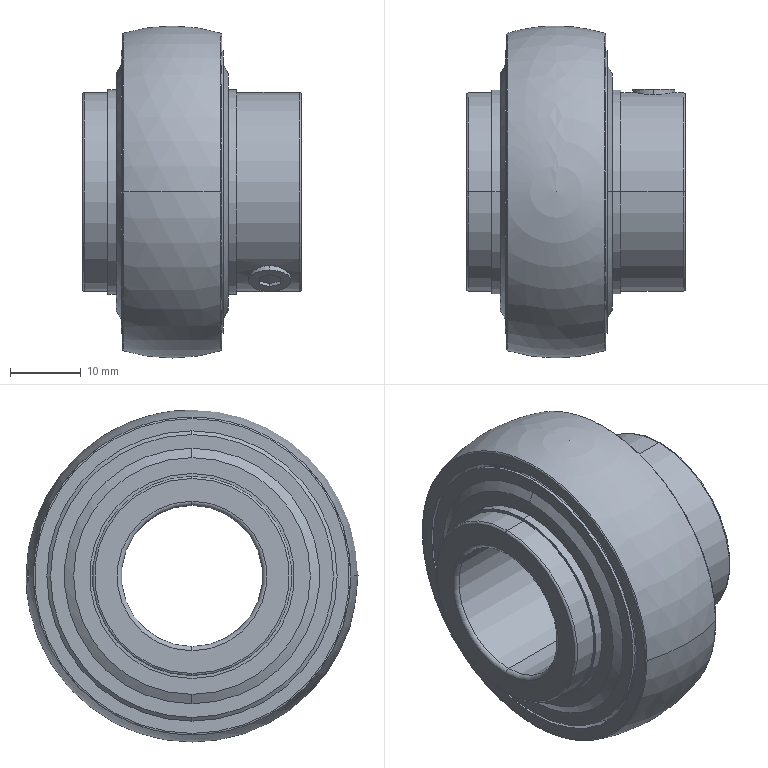Part | SolidWorks | features BaseBody 1 | 1 solid | 184 faces | box 31 x 47 x 47 mm | volume 16946 mm3 | cone 60 | cylinder 46 | plane 42 | torus 34 | sphere 2 | commonest cylinder face diameters 28.2 x14 6 x4 28.994 x4 29.008 x4 29.391 x4 39.85 x4